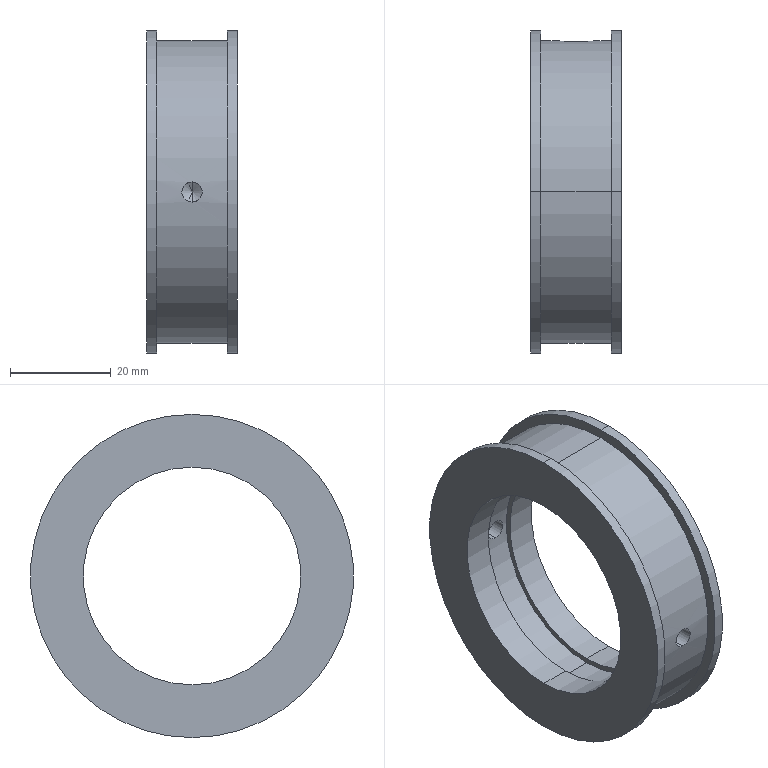Part | SolidWorks | features HoleWzd 3, Fillet 2, Revolution 1 | 1 solid | 31 faces | box 18 x 64 x 64 mm | volume 25166 mm3 | cylinder 18 | plane 7 | torus 2 | spline 2 | cone 2 | commonest cylinder face diameters 4 x4 43.1 x4 64 x4 7.5 x2 45.1 x2 60 x2
STEP:
#1=CARTESIAN_POINT('',(0.6103,28.8,3.75));
#2=VERTEX_POINT('',#1);
#3=CARTESIAN_POINT('',(0.6103,28.8,-3.75));
#4=VERTEX_POINT('',#3);
#5=CARTESIAN_POINT('',(0.6103,28.8,0.));
#6=DIRECTION('',(0.,-1.,0.));
#7=DIRECTION('',(0.,0.,-1.));
#8=AXIS2_PLACEMENT_3D('',#5,#6,#7);
#9=CIRCLE('',#8,3.75);
#10=EDGE_CURVE('',#2,#4,#9,.T.);
#11=ORIENTED_EDGE('',*,*,#10,.F.);
#12=CARTESIAN_POINT('',(0.6103,28.5,3.45));
#13=VERTEX_POINT('',#12);
#14=CARTESIAN_POINT('',(0.6103,28.8,3.45));
#15=DIRECTION('',(1.,0.,0.));
#16=DIRECTION('',(0.,0.,-1.));
#17=AXIS2_PLACEMENT_3D('',#14,#15,#16);
#18=CIRCLE('',#17,0.3);
#19=EDGE_CURVE('',#2,#13,#18,.T.);
#20=ORIENTED_EDGE('',*,*,#19,.T.);
#21=CARTESIAN_POINT('',(0.6103,28.5,-3.45));
#22=VERTEX_POINT('',#21);
#23=CARTESIAN_POINT('',(0.6103,28.5,0.));
#24=DIRECTION('',(0.,1.,0.));
#25=DIRECTION('',(0.,0.,-1.));
#26=AXIS2_PLACEMENT_3D('',#23,#24,#25);
#27=CIRCLE('',#26,3.45);
#28=EDGE_CURVE('',#22,#13,#27,.T.);
#29=ORIENTED_EDGE('',*,*,#28,.F.);
#30=CARTESIAN_POINT('',(0.6103,28.8,-3.45));
#31=DIRECTION('',(-1.,0.,0.));
#32=DIRECTION('',(0.,0.,1.));
#33=AXIS2_PLACEMENT_3D('',#30,#31,#32);
#34=CIRCLE('',#33,0.3);
#35=EDGE_CURVE('',#4,#22,#34,.T.);
#36=ORIENTED_EDGE('',*,*,#35,.F.);
#37=EDGE_LOOP('',(#11,#20,#29,#36));
#38=FACE_OUTER_BOUND('',#37,.T.);
#39=CARTESIAN_POINT('',(0.6103,28.8,0.));
#40=DIRECTION('',(0.,-1.,0.));
#41=DIRECTION('',(0.,0.,-1.));
#42=AXIS2_PLACEMENT_3D('',#39,#40,#41);
#43=TOROIDAL_SURFACE('',#42,3.45,0.3);
#44=ADVANCED_FACE('',(#38),#43,.F.);
#45=CARTESIAN_POINT('',(-0.2424,29.551,-3.652));
#46=VERTEX_POINT('',#45);
#47=CARTESIAN_POINT('',(0.6103,29.537,3.75));
#48=VERTEX_POINT('',#47);
#49=CARTESIAN_POINT('',(-0.2424,29.551,-3.652));
#50=CARTESIAN_POINT('',(-0.4646,29.558,-3.6));
#51=CARTESIAN_POINT('',(-0.6839,29.568,-3.527));
#52=CARTESIAN_POINT('',(-1.101,29.591,-3.345));
#53=CARTESIAN_POINT('',(-1.299,29.605,-3.236));
#54=CARTESIAN_POINT('',(-1.675,29.634,-2.982));
#55=CARTESIAN_POINT('',(-1.854,29.65,-2.836));
#56=CARTESIAN_POINT('',(-2.178,29.682,-2.518));
#57=CARTESIAN_POINT('',(-2.324,29.698,-2.346));
#58=CARTESIAN_POINT('',(-2.586,29.728,-1.974));
#59=CARTESIAN_POINT('',(-2.701,29.742,-1.774));
#60=CARTESIAN_POINT('',(-2.891,29.766,-1.363));
#61=CARTESIAN_POINT('',(-2.967,29.776,-1.149));
#62=CARTESIAN_POINT('',(-3.08,29.792,-0.7059));
#63=CARTESIAN_POINT('',(-3.116,29.797,-0.479));
#64=CARTESIAN_POINT('',(-3.146,29.801,-0.02683));
#65=CARTESIAN_POINT('',(-3.141,29.8,0.2003));
#66=CARTESIAN_POINT('',(-3.089,29.793,0.6567));
#67=CARTESIAN_POINT('',(-3.042,29.786,0.8794));
#68=CARTESIAN_POINT('',(-2.91,29.769,1.312));
#69=CARTESIAN_POINT('',(-2.823,29.757,1.524));
#70=CARTESIAN_POINT('',(-2.613,29.731,1.93));
#71=CARTESIAN_POINT('',(-2.491,29.717,2.121));
#72=CARTESIAN_POINT('',(-2.213,29.686,2.478));
#73=CARTESIAN_POINT('',(-2.056,29.67,2.647));
#74=CARTESIAN_POINT('',(-1.716,29.638,2.95));
#75=CARTESIAN_POINT('',(-1.534,29.623,3.084));
#76=CARTESIAN_POINT('',(-1.147,29.594,3.32));
#77=CARTESIAN_POINT('',(-0.9399,29.581,3.422));
#78=CARTESIAN_POINT('',(-0.5152,29.56,3.584));
#79=CARTESIAN_POINT('',(-0.2972,29.552,3.646));
#80=CARTESIAN_POINT('',(0.1503,29.54,3.729));
#81=CARTESIAN_POINT('',(0.3805,29.537,3.75));
#82=CARTESIAN_POINT('',(0.6103,29.537,3.75));
#83=B_SPLINE_CURVE_WITH_KNOTS('',3,(#49,#50,#51,#52,#53,#54,#55,#56,#57,#58,#59,#60,#61,#62,#63,#64,#65,#66,#67,#68,#69,#70,#71,#72,#73,#74,#75,#76,#77,#78,#79,#80,#81,#82),.UNSPECIFIED.,.F.,.F.,(4,2,2,2,2,2,2,2,2,2,2,2,2,2,2,2,4),(0.01269,0.01337,0.01406,0.01474,0.01543,0.01611,0.0168,0.01748,0.01817,0.01885,0.01954,0.02022,0.02091,0.02159,0.02228,0.02296,0.02365),.UNSPECIFIED.);
#84=EDGE_CURVE('',#46,#48,#83,.T.);
#85=ORIENTED_EDGE('',*,*,#84,.F.);
#86=CARTESIAN_POINT('',(-0.2879,29.749,-3.872));
#87=VERTEX_POINT('',#86);
#88=CARTESIAN_POINT('',(-0.2879,29.551,-3.847));
#89=DIRECTION('',(-0.9734,0.02959,0.2273));
#90=DIRECTION('',(0.2274,0.,0.9738));
#91=AXIS2_PLACEMENT_3D('',#88,#89,#90);
#92=CIRCLE('',#91,0.2);
#93=EDGE_CURVE('',#46,#87,#92,.T.);
#94=ORIENTED_EDGE('',*,*,#93,.T.);
#95=CARTESIAN_POINT('',(1.509,29.749,3.872));
#96=VERTEX_POINT('',#95);
#97=CARTESIAN_POINT('',(1.509,29.749,3.872));
#98=CARTESIAN_POINT('',(1.254,29.741,3.932));
#99=CARTESIAN_POINT('',(0.9958,29.737,3.966));
#100=CARTESIAN_POINT('',(0.4738,29.734,3.983));
#101=CARTESIAN_POINT('',(0.2098,29.737,3.965));
#102=CARTESIAN_POINT('',(-0.3023,29.748,3.878));
#103=CARTESIAN_POINT('',(-0.5513,29.757,3.81));
#104=CARTESIAN_POINT('',(-1.035,29.78,3.624));
#105=CARTESIAN_POINT('',(-1.271,29.795,3.506));
#106=CARTESIAN_POINT('',(-1.707,29.826,3.231));
#107=CARTESIAN_POINT('',(-1.911,29.843,3.072));
#108=CARTESIAN_POINT('',(-2.289,29.878,2.714));
#109=CARTESIAN_POINT('',(-2.459,29.895,2.517));
#110=CARTESIAN_POINT('',(-2.756,29.927,2.096));
#111=CARTESIAN_POINT('',(-2.886,29.943,1.869));
#112=CARTESIAN_POINT('',(-3.098,29.969,1.394));
#113=CARTESIAN_POINT('',(-3.18,29.979,1.149));
#114=CARTESIAN_POINT('',(-3.296,29.994,0.6447));
#115=CARTESIAN_POINT('',(-3.33,29.999,0.3829));
#116=CARTESIAN_POINT('',(-3.346,30.001,-0.135));
#117=CARTESIAN_POINT('',(-3.329,29.999,-0.3927));
#118=CARTESIAN_POINT('',(-3.245,29.987,-0.9056));
#119=CARTESIAN_POINT('',(-3.177,29.979,-1.16));
#120=CARTESIAN_POINT('',(-2.996,29.956,-1.643));
#121=CARTESIAN_POINT('',(-2.882,29.942,-1.876));
#122=CARTESIAN_POINT('',(-2.608,29.911,-2.321));
#123=CARTESIAN_POINT('',(-2.451,29.894,-2.526));
#124=CARTESIAN_POINT('',(-2.1,29.86,-2.904));
#125=CARTESIAN_POINT('',(-1.904,29.842,-3.078));
#126=CARTESIAN_POINT('',(-1.484,29.809,-3.382));
#127=CARTESIAN_POINT('',(-1.261,29.794,-3.512));
#128=CARTESIAN_POINT('',(-0.7903,29.768,-3.727));
#129=CARTESIAN_POINT('',(-0.5411,29.757,-3.813));
#130=CARTESIAN_POINT('',(-0.2879,29.749,-3.872));
#131=B_SPLINE_CURVE_WITH_KNOTS('',3,(#97,#98,#99,#100,#101,#102,#103,#104,#105,#106,#107,#108,#109,#110,#111,#112,#113,#114,#115,#116,#117,#118,#119,#120,#121,#122,#123,#124,#125,#126,#127,#128,#129,#130),.UNSPECIFIED.,.F.,.F.,(4,2,2,2,2,2,2,2,2,2,2,2,2,2,2,2,4),(0.02421,0.025,0.02578,0.02657,0.02735,0.02814,0.02892,0.02971,0.03049,0.03128,0.03206,0.03285,0.03363,0.03442,0.0352,0.03599,0.03677),.UNSPECIFIED.);
#132=EDGE_CURVE('',#96,#87,#131,.T.);
#133=ORIENTED_EDGE('',*,*,#132,.F.);
#134=CARTESIAN_POINT('',(1.463,29.551,3.652));
#135=VERTEX_POINT('',#134);
#136=CARTESIAN_POINT('',(1.509,29.551,3.846));
#137=DIRECTION('',(0.9734,0.02959,-0.2273));
#138=DIRECTION('',(-0.2274,0.,-0.9738));
#139=AXIS2_PLACEMENT_3D('',#136,#137,#138);
#140=CIRCLE('',#139,0.2);
#141=EDGE_CURVE('',#135,#96,#140,.T.);
#142=ORIENTED_EDGE('',*,*,#141,.F.);
#143=CARTESIAN_POINT('',(0.6103,29.537,3.75));
#144=CARTESIAN_POINT('',(0.7544,29.537,3.75));
#145=CARTESIAN_POINT('',(1.041,29.539,3.733));
#146=CARTESIAN_POINT('',(1.323,29.546,3.684));
#147=CARTESIAN_POINT('',(1.463,29.551,3.652));
#148=B_SPLINE_CURVE_WITH_KNOTS('',3,(#143,#144,#145,#146,#147),.UNSPECIFIED.,.F.,.F.,(4,1,4),(0.,0.0004293,0.0008586),.UNSPECIFIED.);
#149=EDGE_CURVE('',#48,#135,#148,.T.);
#150=ORIENTED_EDGE('',*,*,#149,.F.);
#151=EDGE_LOOP('',(#85,#94,#133,#142,#150));
#152=FACE_OUTER_BOUND('',#151,.T.);
#153=CARTESIAN_POINT('',(1.463,29.551,3.652));
#154=CARTESIAN_POINT('',(1.457,29.778,3.653));
#155=CARTESIAN_POINT('',(1.509,29.749,3.872));
#156=CARTESIAN_POINT('',(1.222,29.543,3.708));
#157=CARTESIAN_POINT('',(1.216,29.771,3.709));
#158=CARTESIAN_POINT('',(1.254,29.741,3.932));
#159=CARTESIAN_POINT('',(0.9788,29.538,3.74));
#160=CARTESIAN_POINT('',(0.9757,29.767,3.74));
#161=CARTESIAN_POINT('',(0.9985,29.737,3.966));
#162=CARTESIAN_POINT('',(0.49,29.536,3.756));
#163=CARTESIAN_POINT('',(0.4909,29.765,3.756));
#164=CARTESIAN_POINT('',(0.4835,29.734,3.983));
#165=CARTESIAN_POINT('',(0.2413,29.539,3.74));
#166=CARTESIAN_POINT('',(0.2448,29.767,3.74));
#167=CARTESIAN_POINT('',(0.2217,29.737,3.966));
#168=CARTESIAN_POINT('',(-0.2441,29.55,3.66));
#169=CARTESIAN_POINT('',(-0.237,29.777,3.661));
#170=CARTESIAN_POINT('',(-0.2896,29.748,3.881));
#171=CARTESIAN_POINT('',(-0.4801,29.558,3.596));
#172=CARTESIAN_POINT('',(-0.4712,29.784,3.599));
#173=CARTESIAN_POINT('',(-0.5383,29.757,3.814));
#174=CARTESIAN_POINT('',(-0.9391,29.581,3.424));
#175=CARTESIAN_POINT('',(-0.928,29.804,3.429));
#176=CARTESIAN_POINT('',(-1.022,29.78,3.631));
#177=CARTESIAN_POINT('',(-1.163,29.595,3.313));
#178=CARTESIAN_POINT('',(-1.151,29.817,3.32));
#179=CARTESIAN_POINT('',(-1.257,29.794,3.513));
#180=CARTESIAN_POINT('',(-1.578,29.626,3.055));
#181=CARTESIAN_POINT('',(-1.566,29.844,3.064));
#182=CARTESIAN_POINT('',(-1.695,29.825,3.24));
#183=CARTESIAN_POINT('',(-1.772,29.643,2.907));
#184=CARTESIAN_POINT('',(-1.76,29.859,2.916));
#185=CARTESIAN_POINT('',(-1.899,29.842,3.082));
#186=CARTESIAN_POINT('',(-2.132,29.677,2.57));
#187=CARTESIAN_POINT('',(-2.121,29.89,2.581));
#188=CARTESIAN_POINT('',(-2.278,29.877,2.725));
#189=CARTESIAN_POINT('',(-2.294,29.695,2.384));
#190=CARTESIAN_POINT('',(-2.285,29.905,2.396));
#191=CARTESIAN_POINT('',(-2.449,29.894,2.528));
#192=CARTESIAN_POINT('',(-2.579,29.727,1.988));
#193=CARTESIAN_POINT('',(-2.572,29.934,1.999));
#194=CARTESIAN_POINT('',(-2.749,29.927,2.108));
#195=CARTESIAN_POINT('',(-2.703,29.742,1.774));
#196=CARTESIAN_POINT('',(-2.697,29.948,1.785));
#197=CARTESIAN_POINT('',(-2.88,29.942,1.881));
#198=CARTESIAN_POINT('',(-2.907,29.768,1.325));
#199=CARTESIAN_POINT('',(-2.903,29.971,1.334));
#200=CARTESIAN_POINT('',(-3.094,29.968,1.405));
#201=CARTESIAN_POINT('',(-2.985,29.779,1.093));
#202=CARTESIAN_POINT('',(-2.983,29.981,1.101));
#203=CARTESIAN_POINT('',(-3.177,29.979,1.159));
#204=CARTESIAN_POINT('',(-3.097,29.794,0.6165));
#205=CARTESIAN_POINT('',(-3.096,29.995,0.6213));
#206=CARTESIAN_POINT('',(-3.294,29.994,0.6537));
#207=CARTESIAN_POINT('',(-3.13,29.799,0.3687));
#208=CARTESIAN_POINT('',(-3.129,29.999,0.3714));
#209=CARTESIAN_POINT('',(-3.329,29.999,0.391));
#210=CARTESIAN_POINT('',(-3.146,29.801,-0.1217));
#211=CARTESIAN_POINT('',(-3.146,30.001,-0.1225));
#212=CARTESIAN_POINT('',(-3.346,30.001,-0.129));
#213=CARTESIAN_POINT('',(-3.13,29.799,-0.3657));
#214=CARTESIAN_POINT('',(-3.13,29.999,-0.3686));
#215=CARTESIAN_POINT('',(-3.329,29.999,-0.3878));
#216=CARTESIAN_POINT('',(-3.05,29.788,-0.8512));
#217=CARTESIAN_POINT('',(-3.049,29.989,-0.8574));
#218=CARTESIAN_POINT('',(-3.245,29.988,-0.9027));
#219=CARTESIAN_POINT('',(-2.986,29.779,-1.092));
#220=CARTESIAN_POINT('',(-2.983,29.981,-1.1));
#221=CARTESIAN_POINT('',(-3.177,29.979,-1.158));
#222=CARTESIAN_POINT('',(-2.813,29.756,-1.549));
#223=CARTESIAN_POINT('',(-2.809,29.96,-1.559));
#224=CARTESIAN_POINT('',(-2.996,29.956,-1.643));
#225=CARTESIAN_POINT('',(-2.705,29.743,-1.769));
#226=CARTESIAN_POINT('',(-2.699,29.948,-1.78));
#227=CARTESIAN_POINT('',(-2.882,29.942,-1.876));
#228=CARTESIAN_POINT('',(-2.444,29.711,-2.189));
#229=CARTESIAN_POINT('',(-2.436,29.92,-2.201));
#230=CARTESIAN_POINT('',(-2.607,29.911,-2.322));
#231=CARTESIAN_POINT('',(-2.295,29.695,-2.383));
#232=CARTESIAN_POINT('',(-2.286,29.905,-2.395));
#233=CARTESIAN_POINT('',(-2.45,29.894,-2.527));
#234=CARTESIAN_POINT('',(-1.962,29.661,-2.74));
#235=CARTESIAN_POINT('',(-1.95,29.875,-2.751));
#236=CARTESIAN_POINT('',(-2.099,29.86,-2.905));
#237=CARTESIAN_POINT('',(-1.775,29.643,-2.904));
#238=CARTESIAN_POINT('',(-1.763,29.859,-2.914));
#239=CARTESIAN_POINT('',(-1.902,29.842,-3.08));
#240=CARTESIAN_POINT('',(-1.376,29.61,-3.19));
#241=CARTESIAN_POINT('',(-1.364,29.83,-3.198));
#242=CARTESIAN_POINT('',(-1.482,29.809,-3.383));
#243=CARTESIAN_POINT('',(-1.165,29.595,-3.312));
#244=CARTESIAN_POINT('',(-1.153,29.817,-3.319));
#245=CARTESIAN_POINT('',(-1.259,29.794,-3.512));
#246=CARTESIAN_POINT('',(-0.7184,29.569,-3.515));
#247=CARTESIAN_POINT('',(-0.7081,29.794,-3.519));
#248=CARTESIAN_POINT('',(-0.7893,29.768,-3.728));
#249=CARTESIAN_POINT('',(-0.4816,29.558,-3.596));
#250=CARTESIAN_POINT('',(-0.4729,29.784,-3.598));
#251=CARTESIAN_POINT('',(-0.5398,29.757,-3.813));
#252=CARTESIAN_POINT('',(-0.2424,29.551,-3.652));
#253=CARTESIAN_POINT('',(-0.2359,29.778,-3.653));
#254=CARTESIAN_POINT('',(-0.2879,29.749,-3.872));
#255=(BOUNDED_SURFACE()B_SPLINE_SURFACE(3,2,((#153,#154,#155),(#156,#157,#158),(#159,#160,#161),(#162,#163,#164),(#165,#166,#167),(#168,#169,#170),(#171,#172,#173),(#174,#175,#176),(#177,#178,#179),(#180,#181,#182),(#183,#184,#185),(#186,#187,#188),(#189,#190,#191),(#192,#193,#194),(#195,#196,#197),(#198,#199,#200),(#201,#202,#203),(#204,#205,#206),(#207,#208,#209),(#210,#211,#212),(#213,#214,#215),(#216,#217,#218),(#219,#220,#221),(#222,#223,#224),(#225,#226,#227),(#228,#229,#230),(#231,#232,#233),(#234,#235,#236),(#237,#238,#239),(#240,#241,#242),(#243,#244,#245),(#246,#247,#248),(#249,#250,#251),(#252,#253,#254)),.UNSPECIFIED.,.F.,.F.,.F.)B_SPLINE_SURFACE_WITH_KNOTS((4,2,2,2,2,2,2,2,2,2,2,2,2,2,2,2,4),(3,3),(0.,0.0007725,0.001545,0.002318,0.00309,0.003863,0.004635,0.005408,0.00618,0.006953,0.007725,0.008498,0.00927,0.01004,0.01082,0.01159,0.01236),(0.,1.),.UNSPECIFIED.)GEOMETRIC_REPRESENTATION_ITEM()RATIONAL_B_SPLINE_SURFACE(((1.,0.6612,1.),(1.,0.6597,1.),(1.,0.6588,1.),(1.,0.6584,1.),(1.,0.6589,1.),(1.,0.661,1.),(1.,0.6626,1.),(1.,0.6669,1.),(1.,0.6696,1.),(1.,0.6754,1.),(1.,0.6785,1.),(1.,0.6849,1.),(1.,0.688,1.),(1.,0.694,1.),(1.,0.6967,1.),(1.,0.7014,1.),(1.,0.7033,1.),(1.,0.706,1.),(1.,0.7069,1.),(1.,0.7073,1.),(1.,0.7069,1.),(1.,0.7049,1.),(1.,0.7033,1.),(1.,0.6992,1.),(1.,0.6968,1.),(1.,0.6911,1.),(1.,0.688,1.),(1.,0.6817,1.),(1.,0.6785,1.),(1.,0.6724,1.),(1.,0.6696,1.),(1.,0.6647,1.),(1.,0.6626,1.),(1.,0.6612,1.)))REPRESENTATION_ITEM('')SURFACE());
#256=ADVANCED_FACE('',(#152),#255,.T.);
#257=CARTESIAN_POINT('',(0.6103,-24.798,0.));
#258=VERTEX_POINT('',#257);
#259=CARTESIAN_POINT('',(0.6103,-26.,-2.));
#260=VERTEX_POINT('',#259);
#261=CARTESIAN_POINT('',(0.6103,-26.,-2.));
#262=DIRECTION('',(0.,-0.515,-0.8572));
#263=VECTOR('',#262,1000.);
#264=LINE('',#261,#263);
#265=EDGE_CURVE('',#258,#260,#264,.T.);
#266=ORIENTED_EDGE('',*,*,#265,.F.);
#267=CARTESIAN_POINT('',(0.6103,-26.,2.));
#268=VERTEX_POINT('',#267);
#269=CARTESIAN_POINT('',(0.6103,-26.,2.));
#270=DIRECTION('',(0.,-0.515,0.8572));
#271=VECTOR('',#270,1000.);
#272=LINE('',#269,#271);
#273=EDGE_CURVE('',#258,#268,#272,.T.);
#274=ORIENTED_EDGE('',*,*,#273,.T.);
#275=CARTESIAN_POINT('',(0.6103,-26.,0.));
#276=DIRECTION('',(0.,-1.,0.));
#277=DIRECTION('',(0.,0.,-1.));
#278=AXIS2_PLACEMENT_3D('',#275,#276,#277);
#279=CIRCLE('',#278,2.);
#280=EDGE_CURVE('',#268,#260,#279,.T.);
#281=ORIENTED_EDGE('',*,*,#280,.T.);
#282=EDGE_LOOP('',(#266,#274,#281));
#283=FACE_OUTER_BOUND('',#282,.T.);
#284=CARTESIAN_POINT('',(0.6103,-26.,0.));
#285=DIRECTION('',(0.,-1.,0.));
#286=DIRECTION('',(0.,0.,-1.));
#287=AXIS2_PLACEMENT_3D('',#284,#285,#286);
#288=CONICAL_SURFACE('',#287,2.,1.03);
#289=ADVANCED_FACE('',(#283),#288,.F.);
#290=ORIENTED_EDGE('',*,*,#280,.F.);
#291=CARTESIAN_POINT('',(0.6103,-29.933,2.));
#292=VERTEX_POINT('',#291);
#293=CARTESIAN_POINT('',(0.6103,-30.,2.));
#294=DIRECTION('',(0.,-1.,0.));
#295=VECTOR('',#294,1000.);
#296=LINE('',#293,#295);
#297=EDGE_CURVE('',#268,#292,#296,.T.);
#298=ORIENTED_EDGE('',*,*,#297,.T.);
#299=CARTESIAN_POINT('',(0.6103,-29.933,-2.));
#300=VERTEX_POINT('',#299);
#301=CARTESIAN_POINT('',(0.6103,-29.933,-2.));
#302=CARTESIAN_POINT('',(0.4782,-29.933,-2.));
#303=CARTESIAN_POINT('',(0.3482,-29.934,-1.987));
#304=CARTESIAN_POINT('',(0.0925,-29.937,-1.936));
#305=CARTESIAN_POINT('',(-0.03454,-29.94,-1.898));
#306=CARTESIAN_POINT('',(-0.2768,-29.946,-1.797));
#307=CARTESIAN_POINT('',(-0.3916,-29.95,-1.736));
#308=CARTESIAN_POINT('',(-0.609,-29.958,-1.591));
#309=CARTESIAN_POINT('',(-0.7119,-29.962,-1.506));
#310=CARTESIAN_POINT('',(-0.9886,-29.975,-1.229));
#311=CARTESIAN_POINT('',(-1.138,-29.984,-1.006));
#312=CARTESIAN_POINT('',(-1.337,-29.996,-0.525));
#313=CARTESIAN_POINT('',(-1.39,-30.,-0.2617));
#314=CARTESIAN_POINT('',(-1.39,-30.,0.1298));
#315=CARTESIAN_POINT('',(-1.377,-29.999,0.2623));
#316=CARTESIAN_POINT('',(-1.326,-29.996,0.5189));
#317=CARTESIAN_POINT('',(-1.288,-29.993,0.6436));
#318=CARTESIAN_POINT('',(-1.188,-29.987,0.8858));
#319=CARTESIAN_POINT('',(-1.125,-29.983,1.003));
#320=CARTESIAN_POINT('',(-0.9802,-29.975,1.22));
#321=CARTESIAN_POINT('',(-0.8975,-29.971,1.321));
#322=CARTESIAN_POINT('',(-0.7108,-29.962,1.507));
#323=CARTESIAN_POINT('',(-0.6097,-29.958,1.59));
#324=CARTESIAN_POINT('',(-0.3931,-29.95,1.735));
#325=CARTESIAN_POINT('',(-0.2762,-29.946,1.798));
#326=CARTESIAN_POINT('',(-0.03384,-29.94,1.898));
#327=CARTESIAN_POINT('',(0.09085,-29.937,1.936));
#328=CARTESIAN_POINT('',(0.3472,-29.934,1.987));
#329=CARTESIAN_POINT('',(0.4798,-29.933,2.));
#330=CARTESIAN_POINT('',(0.6103,-29.933,2.));
#331=B_SPLINE_CURVE_WITH_KNOTS('',3,(#301,#302,#303,#304,#305,#306,#307,#308,#309,#310,#311,#312,#313,#314,#315,#316,#317,#318,#319,#320,#321,#322,#323,#324,#325,#326,#327,#328,#329,#330),.UNSPECIFIED.,.F.,.F.,(4,2,2,2,2,2,2,2,2,2,2,2,2,2,4),(0.,0.0003909,0.0007818,0.001173,0.001564,0.002345,0.003127,0.003518,0.003909,0.0043,0.004691,0.005082,0.005473,0.005864,0.006255),.UNSPECIFIED.);
#332=EDGE_CURVE('',#300,#292,#331,.T.);
#333=ORIENTED_EDGE('',*,*,#332,.F.);
#334=CARTESIAN_POINT('',(0.6103,-30.,-2.));
#335=DIRECTION('',(0.,-1.,0.));
#336=VECTOR('',#335,1000.);
#337=LINE('',#334,#336);
#338=EDGE_CURVE('',#260,#300,#337,.T.);
#339=ORIENTED_EDGE('',*,*,#338,.F.);
#340=EDGE_LOOP('',(#290,#298,#333,#339));
#341=FACE_OUTER_BOUND('',#340,.T.);
#342=CARTESIAN_POINT('',(0.6103,-30.,0.));
#343=DIRECTION('',(0.,-1.,0.));
#344=DIRECTION('',(0.,0.,-1.));
#345=AXIS2_PLACEMENT_3D('',#342,#343,#344);
#346=CYLINDRICAL_SURFACE('',#345,2.);
#347=ADVANCED_FACE('',(#341),#346,.F.);
#348=CARTESIAN_POINT('',(0.6103,22.461,-2.));
#349=VERTEX_POINT('',#348);
#350=CARTESIAN_POINT('',(0.6103,22.461,2.));
#351=VERTEX_POINT('',#350);
#352=CARTESIAN_POINT('',(0.6103,22.461,-2.));
#353=CARTESIAN_POINT('',(0.3493,22.461,-2.));
#354=CARTESIAN_POINT('',(0.08608,22.466,-1.948));
#355=CARTESIAN_POINT('',(-0.3953,22.482,-1.748));
#356=CARTESIAN_POINT('',(-0.6184,22.494,-1.599));
#357=CARTESIAN_POINT('',(-0.8951,22.511,-1.323));
#358=CARTESIAN_POINT('',(-0.9796,22.517,-1.22));
#359=CARTESIAN_POINT('',(-1.125,22.528,-1.003));
#360=CARTESIAN_POINT('',(-1.186,22.533,-0.8882));
#361=CARTESIAN_POINT('',(-1.287,22.541,-0.6463));
#362=CARTESIAN_POINT('',(-1.325,22.544,-0.5192));
#363=CARTESIAN_POINT('',(-1.377,22.549,-0.2635));
#364=CARTESIAN_POINT('',(-1.39,22.55,-0.1336));
#365=CARTESIAN_POINT('',(-1.39,22.55,0.1305));
#366=CARTESIAN_POINT('',(-1.377,22.549,0.2608));
#367=CARTESIAN_POINT('',(-1.326,22.544,0.5164));
#368=CARTESIAN_POINT('',(-1.288,22.541,0.6434));
#369=CARTESIAN_POINT('',(-1.188,22.533,0.8857));
#370=CARTESIAN_POINT('',(-1.126,22.528,1.001));
#371=CARTESIAN_POINT('',(-0.9814,22.517,1.218));
#372=CARTESIAN_POINT('',(-0.897,22.511,1.321));
#373=CARTESIAN_POINT('',(-0.6205,22.494,1.598));
#374=CARTESIAN_POINT('',(-0.3977,22.482,1.747));
#375=CARTESIAN_POINT('',(0.08333,22.466,1.947));
#376=CARTESIAN_POINT('',(0.346,22.461,2.));
#377=CARTESIAN_POINT('',(0.6103,22.461,2.));
#378=B_SPLINE_CURVE_WITH_KNOTS('',3,(#352,#353,#354,#355,#356,#357,#358,#359,#360,#361,#362,#363,#364,#365,#366,#367,#368,#369,#370,#371,#372,#373,#374,#375,#376,#377),.UNSPECIFIED.,.F.,.F.,(4,2,2,2,2,2,2,2,2,2,2,2,4),(0.006256,0.007038,0.00782,0.008211,0.008601,0.008992,0.009383,0.009774,0.01017,0.01056,0.01095,0.01173,0.01251),.UNSPECIFIED.);
#379=EDGE_CURVE('',#349,#351,#378,.T.);
#380=ORIENTED_EDGE('',*,*,#379,.F.);
#381=CARTESIAN_POINT('',(0.6103,28.5,-2.));
#382=VERTEX_POINT('',#381);
#383=CARTESIAN_POINT('',(0.6103,28.5,-2.));
#384=DIRECTION('',(0.,1.,0.));
#385=VECTOR('',#384,1000.);
#386=LINE('',#383,#385);
#387=EDGE_CURVE('',#349,#382,#386,.T.);
#388=ORIENTED_EDGE('',*,*,#387,.T.);
#389=CARTESIAN_POINT('',(0.6103,28.5,2.));
#390=VERTEX_POINT('',#389);
#391=CARTESIAN_POINT('',(0.6103,28.5,0.));
#392=DIRECTION('',(0.,1.,0.));
#393=DIRECTION('',(0.,0.,1.));
#394=AXIS2_PLACEMENT_3D('',#391,#392,#393);
#395=CIRCLE('',#394,2.);
#396=EDGE_CURVE('',#382,#390,#395,.T.);
#397=ORIENTED_EDGE('',*,*,#396,.T.);
#398=CARTESIAN_POINT('',(0.6103,28.5,2.));
#399=DIRECTION('',(0.,1.,0.));
#400=VECTOR('',#399,1000.);
#401=LINE('',#398,#400);
#402=EDGE_CURVE('',#351,#390,#401,.T.);
#403=ORIENTED_EDGE('',*,*,#402,.F.);
#404=EDGE_LOOP('',(#380,#388,#397,#403));
#405=FACE_OUTER_BOUND('',#404,.T.);
#406=CARTESIAN_POINT('',(0.6103,28.5,0.));
#407=DIRECTION('',(0.,1.,0.));
#408=DIRECTION('',(0.,0.,1.));
#409=AXIS2_PLACEMENT_3D('',#406,#407,#408);
#410=CYLINDRICAL_SURFACE('',#409,2.);
#411=ADVANCED_FACE('',(#405),#410,.F.);
#412=ORIENTED_EDGE('',*,*,#10,.T.);
#413=CARTESIAN_POINT('',(0.6103,29.537,-3.75));
#414=VERTEX_POINT('',#413);
#415=CARTESIAN_POINT('',(0.6103,30.,-3.75));
#416=DIRECTION('',(0.,1.,0.));
#417=VECTOR('',#416,1000.);
#418=LINE('',#415,#417);
#419=EDGE_CURVE('',#4,#414,#418,.T.);
#420=ORIENTED_EDGE('',*,*,#419,.T.);
#421=CARTESIAN_POINT('',(0.6103,29.537,-3.75));
#422=CARTESIAN_POINT('',(0.4679,29.537,-3.75));
#423=CARTESIAN_POINT('',(0.325,29.538,-3.742));
#424=CARTESIAN_POINT('',(0.03842,29.543,-3.709));
#425=CARTESIAN_POINT('',(-0.1029,29.546,-3.684));
#426=CARTESIAN_POINT('',(-0.2424,29.551,-3.652));
#427=B_SPLINE_CURVE_WITH_KNOTS('',3,(#421,#422,#423,#424,#425,#426),.UNSPECIFIED.,.F.,.F.,(4,2,4),(0.01183,0.01226,0.01269),.UNSPECIFIED.);
#428=EDGE_CURVE('',#414,#46,#427,.T.);
#429=ORIENTED_EDGE('',*,*,#428,.T.);
#430=ORIENTED_EDGE('',*,*,#84,.T.);
#431=CARTESIAN_POINT('',(0.6103,30.,3.75));
#432=DIRECTION('',(0.,1.,0.));
#433=VECTOR('',#432,1000.);
#434=LINE('',#431,#433);
#435=EDGE_CURVE('',#2,#48,#434,.T.);
#436=ORIENTED_EDGE('',*,*,#435,.F.);
#437=EDGE_LOOP('',(#412,#420,#429,#430,#436));
#438=FACE_OUTER_BOUND('',#437,.T.);
#439=CARTESIAN_POINT('',(0.6103,30.,0.));
#440=DIRECTION('',(0.,1.,0.));
#441=DIRECTION('',(0.,0.,1.));
#442=AXIS2_PLACEMENT_3D('',#439,#440,#441);
#443=CYLINDRICAL_SURFACE('',#442,3.75);
#444=ADVANCED_FACE('',(#438),#443,.F.);
#445=CARTESIAN_POINT('',(-2.39,0.,-21.55));
#446=VERTEX_POINT('',#445);
#447=CARTESIAN_POINT('',(-2.39,0.,21.55));
#448=VERTEX_POINT('',#447);
#449=CARTESIAN_POINT('',(-2.39,0.,0.));
#450=DIRECTION('',(-1.,0.,0.));
#451=DIRECTION('',(0.,0.,1.));
#452=AXIS2_PLACEMENT_3D('',#449,#450,#451);
#453=CIRCLE('',#452,21.55);
#454=EDGE_CURVE('',#446,#448,#453,.T.);
#455=ORIENTED_EDGE('',*,*,#454,.F.);
#456=CARTESIAN_POINT('',(-8.39,0.,-21.55));
#457=VERTEX_POINT('',#456);
#458=CARTESIAN_POINT('',(-19.037,0.,-21.55));
#459=DIRECTION('',(-1.,0.,0.));
#460=VECTOR('',#459,1000.);
#461=LINE('',#458,#460);
#462=EDGE_CURVE('',#446,#457,#461,.T.);
#463=ORIENTED_EDGE('',*,*,#462,.T.);
#464=CARTESIAN_POINT('',(-8.39,0.,21.55));
#465=VERTEX_POINT('',#464);
#466=CARTESIAN_POINT('',(-8.39,0.,0.));
#467=DIRECTION('',(-1.,0.,0.));
#468=DIRECTION('',(0.,0.,1.));
#469=AXIS2_PLACEMENT_3D('',#466,#467,#468);
#470=CIRCLE('',#469,21.55);
#471=EDGE_CURVE('',#457,#465,#470,.T.);
#472=ORIENTED_EDGE('',*,*,#471,.T.);
#473=CARTESIAN_POINT('',(-19.037,0.,21.55));
#474=DIRECTION('',(-1.,0.,0.));
#475=VECTOR('',#474,1000.);
#476=LINE('',#473,#475);
#477=EDGE_CURVE('',#448,#465,#476,.T.);
#478=ORIENTED_EDGE('',*,*,#477,.F.);
#479=EDGE_LOOP('',(#455,#463,#472,#478));
#480=FACE_OUTER_BOUND('',#479,.T.);
#481=CARTESIAN_POINT('',(-19.037,0.,0.));
#482=DIRECTION('',(-1.,0.,0.));
#483=DIRECTION('',(0.,0.,1.));
#484=AXIS2_PLACEMENT_3D('',#481,#482,#483);
#485=CYLINDRICAL_SURFACE('',#484,21.55);
#486=ADVANCED_FACE('',(#480),#485,.F.);
#487=CARTESIAN_POINT('',(3.61,0.,-22.55));
#488=VERTEX_POINT('',#487);
#489=CARTESIAN_POINT('',(3.61,0.,22.55));
#490=VERTEX_POINT('',#489);
#491=CARTESIAN_POINT('',(3.61,0.,0.));
#492=DIRECTION('',(-1.,0.,0.));
#493=DIRECTION('',(0.,0.,1.));
#494=AXIS2_PLACEMENT_3D('',#491,#492,#493);
#495=CIRCLE('',#494,22.55);
#496=EDGE_CURVE('',#488,#490,#495,.T.);
#497=ORIENTED_EDGE('',*,*,#496,.F.);
#498=CARTESIAN_POINT('',(-2.39,0.,-22.55));
#499=VERTEX_POINT('',#498);
#500=CARTESIAN_POINT('',(-19.037,0.,-22.55));
#501=DIRECTION('',(-1.,0.,0.));
#502=VECTOR('',#501,1000.);
#503=LINE('',#500,#502);
#504=EDGE_CURVE('',#488,#499,#503,.T.);
#505=ORIENTED_EDGE('',*,*,#504,.T.);
#506=CARTESIAN_POINT('',(-2.39,0.,22.55));
#507=VERTEX_POINT('',#506);
#508=CARTESIAN_POINT('',(-2.39,0.,0.));
#509=DIRECTION('',(-1.,0.,0.));
#510=DIRECTION('',(0.,0.,1.));
#511=AXIS2_PLACEMENT_3D('',#508,#509,#510);
#512=CIRCLE('',#511,22.55);
#513=EDGE_CURVE('',#499,#507,#512,.T.);
#514=ORIENTED_EDGE('',*,*,#513,.T.);
#515=CARTESIAN_POINT('',(-19.037,0.,22.55));
#516=DIRECTION('',(-1.,0.,0.));
#517=VECTOR('',#516,1000.);
#518=LINE('',#515,#517);
#519=EDGE_CURVE('',#490,#507,#518,.T.);
#520=ORIENTED_EDGE('',*,*,#519,.F.);
#521=EDGE_LOOP('',(#497,#505,#514,#520));
#522=FACE_OUTER_BOUND('',#521,.T.);
#523=CARTESIAN_POINT('',(-19.037,0.,0.));
#524=DIRECTION('',(-1.,0.,0.));
#525=DIRECTION('',(0.,0.,1.));
#526=AXIS2_PLACEMENT_3D('',#523,#524,#525);
#527=CYLINDRICAL_SURFACE('',#526,22.55);
#528=ADVANCED_FACE('',(#522),#527,.F.);
#529=CARTESIAN_POINT('',(9.61,0.,-21.55));
#530=VERTEX_POINT('',#529);
#531=CARTESIAN_POINT('',(9.61,0.,21.55));
#532=VERTEX_POINT('',#531);
#533=CARTESIAN_POINT('',(9.61,0.,0.));
#534=DIRECTION('',(-1.,0.,0.));
#535=DIRECTION('',(0.,0.,1.));
#536=AXIS2_PLACEMENT_3D('',#533,#534,#535);
#537=CIRCLE('',#536,21.55);
#538=EDGE_CURVE('',#530,#532,#537,.T.);
#539=ORIENTED_EDGE('',*,*,#538,.F.);
#540=CARTESIAN_POINT('',(3.61,0.,-21.55));
#541=VERTEX_POINT('',#540);
#542=CARTESIAN_POINT('',(-19.037,0.,-21.55));
#543=DIRECTION('',(-1.,0.,0.));
#544=VECTOR('',#543,1000.);
#545=LINE('',#542,#544);
#546=EDGE_CURVE('',#530,#541,#545,.T.);
#547=ORIENTED_EDGE('',*,*,#546,.T.);
#548=CARTESIAN_POINT('',(3.61,0.,21.55));
#549=VERTEX_POINT('',#548);
#550=CARTESIAN_POINT('',(3.61,0.,0.));
#551=DIRECTION('',(-1.,0.,0.));
#552=DIRECTION('',(0.,0.,1.));
#553=AXIS2_PLACEMENT_3D('',#550,#551,#552);
#554=CIRCLE('',#553,21.55);
#555=EDGE_CURVE('',#541,#549,#554,.T.);
#556=ORIENTED_EDGE('',*,*,#555,.T.);
#557=CARTESIAN_POINT('',(-19.037,0.,21.55));
#558=DIRECTION('',(-1.,0.,0.));
#559=VECTOR('',#558,1000.);
#560=LINE('',#557,#559);
#561=EDGE_CURVE('',#532,#549,#560,.T.);
#562=ORIENTED_EDGE('',*,*,#561,.F.);
#563=EDGE_LOOP('',(#539,#547,#556,#562));
#564=FACE_OUTER_BOUND('',#563,.T.);
#565=CARTESIAN_POINT('',(-19.037,0.,0.));
#566=DIRECTION('',(-1.,0.,0.));
#567=DIRECTION('',(0.,0.,1.));
#568=AXIS2_PLACEMENT_3D('',#565,#566,#567);
#569=CYLINDRICAL_SURFACE('',#568,21.55);
#570=ADVANCED_FACE('',(#564),#569,.F.);
#571=CARTESIAN_POINT('',(9.61,0.,32.));
#572=VERTEX_POINT('',#571);
#573=CARTESIAN_POINT('',(9.61,0.,-32.));
#574=VERTEX_POINT('',#573);
#575=CARTESIAN_POINT('',(9.61,0.,0.));
#576=DIRECTION('',(-1.,0.,0.));
#577=DIRECTION('',(0.,0.,1.));
#578=AXIS2_PLACEMENT_3D('',#575,#576,#577);
#579=CIRCLE('',#578,32.);
#580=EDGE_CURVE('',#572,#574,#579,.T.);
#581=ORIENTED_EDGE('',*,*,#580,.T.);
#582=CARTESIAN_POINT('',(7.61,0.,-32.));
#583=VERTEX_POINT('',#582);
#584=CARTESIAN_POINT('',(-19.037,0.,-32.));
#585=DIRECTION('',(-1.,0.,0.));
#586=VECTOR('',#585,1000.);
#587=LINE('',#584,#586);
#588=EDGE_CURVE('',#574,#583,#587,.T.);
#589=ORIENTED_EDGE('',*,*,#588,.T.);
#590=CARTESIAN_POINT('',(7.61,0.,32.));
#591=VERTEX_POINT('',#590);
#592=CARTESIAN_POINT('',(7.61,0.,0.));
#593=DIRECTION('',(-1.,0.,0.));
#594=DIRECTION('',(0.,0.,1.));
#595=AXIS2_PLACEMENT_3D('',#592,#593,#594);
#596=CIRCLE('',#595,32.);
#597=EDGE_CURVE('',#591,#583,#596,.T.);
#598=ORIENTED_EDGE('',*,*,#597,.F.);
#599=CARTESIAN_POINT('',(-19.037,0.,32.));
#600=DIRECTION('',(-1.,0.,0.));
#601=VECTOR('',#600,1000.);
#602=LINE('',#599,#601);
#603=EDGE_CURVE('',#572,#591,#602,.T.);
#604=ORIENTED_EDGE('',*,*,#603,.F.);
#605=EDGE_LOOP('',(#581,#589,#598,#604));
#606=FACE_OUTER_BOUND('',#605,.T.);
#607=CARTESIAN_POINT('',(-19.037,0.,0.));
#608=DIRECTION('',(-1.,0.,0.));
#609=DIRECTION('',(0.,0.,1.));
#610=AXIS2_PLACEMENT_3D('',#607,#608,#609);
#611=CYLINDRICAL_SURFACE('',#610,32.);
#612=ADVANCED_FACE('',(#606),#611,.T.);
#613=ORIENTED_EDGE('',*,*,#132,.T.);
#614=CARTESIAN_POINT('',(-0.2879,29.749,-3.872));
#615=CARTESIAN_POINT('',(-0.03455,29.741,-3.932));
#616=CARTESIAN_POINT('',(0.2272,29.737,-3.966));
#617=CARTESIAN_POINT('',(0.7456,29.734,-3.983));
#618=CARTESIAN_POINT('',(1.003,29.737,-3.965));
#619=CARTESIAN_POINT('',(1.516,29.748,-3.879));
#620=CARTESIAN_POINT('',(1.77,29.757,-3.81));
#621=CARTESIAN_POINT('',(2.253,29.78,-3.626));
#622=CARTESIAN_POINT('',(2.484,29.794,-3.51));
#623=CARTESIAN_POINT('',(2.927,29.826,-3.232));
#624=CARTESIAN_POINT('',(3.131,29.843,-3.073));
#625=CARTESIAN_POINT('',(3.505,29.877,-2.718));
#626=CARTESIAN_POINT('',(3.677,29.895,-2.519));
#627=CARTESIAN_POINT('',(3.977,29.927,-2.096));
#628=CARTESIAN_POINT('',(4.105,29.942,-1.872));
#629=CARTESIAN_POINT('',(4.317,29.968,-1.399));
#630=CARTESIAN_POINT('',(4.401,29.979,-1.149));
#631=CARTESIAN_POINT('',(4.517,29.994,-0.6445));
#632=CARTESIAN_POINT('',(4.55,29.999,-0.3881));
#633=CARTESIAN_POINT('',(4.567,30.001,0.1335));
#634=CARTESIAN_POINT('',(4.549,29.998,0.3946));
#635=CARTESIAN_POINT('',(4.465,29.987,0.9045));
#636=CARTESIAN_POINT('',(4.398,29.979,1.157));
#637=CARTESIAN_POINT('',(4.216,29.956,1.646));
#638=CARTESIAN_POINT('',(4.102,29.942,1.877));
#639=CARTESIAN_POINT('',(3.831,29.911,2.317));
#640=CARTESIAN_POINT('',(3.671,29.894,2.527));
#641=CARTESIAN_POINT('',(3.319,29.86,2.906));
#642=CARTESIAN_POINT('',(3.126,29.842,3.077));
#643=CARTESIAN_POINT('',(2.705,29.809,3.381));
#644=CARTESIAN_POINT('',(2.478,29.794,3.514));
#645=CARTESIAN_POINT('',(2.008,29.768,3.728));
#646=CARTESIAN_POINT('',(1.764,29.757,3.812));
#647=CARTESIAN_POINT('',(1.509,29.749,3.872));
#648=B_SPLINE_CURVE_WITH_KNOTS('',3,(#614,#615,#616,#617,#618,#619,#620,#621,#622,#623,#624,#625,#626,#627,#628,#629,#630,#631,#632,#633,#634,#635,#636,#637,#638,#639,#640,#641,#642,#643,#644,#645,#646,#647),.UNSPECIFIED.,.F.,.F.,(4,2,2,2,2,2,2,2,2,2,2,2,2,2,2,2,4),(0.01165,0.01243,0.01322,0.014,0.01479,0.01557,0.01636,0.01714,0.01793,0.01872,0.0195,0.02029,0.02107,0.02186,0.02264,0.02343,0.02421),.UNSPECIFIED.);
#649=EDGE_CURVE('',#87,#96,#648,.T.);
#650=ORIENTED_EDGE('',*,*,#649,.T.);
#651=EDGE_LOOP('',(#613,#650));
#652=FACE_BOUND('',#651,.T.);
#653=CARTESIAN_POINT('',(7.61,0.,30.));
#654=VERTEX_POINT('',#653);
#655=CARTESIAN_POINT('',(7.61,0.,-30.));
#656=VERTEX_POINT('',#655);
#657=CARTESIAN_POINT('',(7.61,0.,0.));
#658=DIRECTION('',(-1.,0.,0.));
#659=DIRECTION('',(0.,0.,1.));
#660=AXIS2_PLACEMENT_3D('',#657,#658,#659);
#661=CIRCLE('',#660,30.);
#662=EDGE_CURVE('',#654,#656,#661,.T.);
#663=ORIENTED_EDGE('',*,*,#662,.T.);
#664=CARTESIAN_POINT('',(-6.39,0.,-30.));
#665=VERTEX_POINT('',#664);
#666=CARTESIAN_POINT('',(-19.037,0.,-30.));
#667=DIRECTION('',(-1.,0.,0.));
#668=VECTOR('',#667,1000.);
#669=LINE('',#666,#668);
#670=EDGE_CURVE('',#656,#665,#669,.T.);
#671=ORIENTED_EDGE('',*,*,#670,.T.);
#672=CARTESIAN_POINT('',(-6.39,0.,30.));
#673=VERTEX_POINT('',#672);
#674=CARTESIAN_POINT('',(-6.39,0.,0.));
#675=DIRECTION('',(-1.,0.,0.));
#676=DIRECTION('',(0.,0.,1.));
#677=AXIS2_PLACEMENT_3D('',#674,#675,#676);
#678=CIRCLE('',#677,30.);
#679=EDGE_CURVE('',#673,#665,#678,.T.);
#680=ORIENTED_EDGE('',*,*,#679,.F.);
#681=CARTESIAN_POINT('',(-19.037,0.,30.));
#682=DIRECTION('',(-1.,0.,0.));
#683=VECTOR('',#682,1000.);
#684=LINE('',#681,#683);
#685=EDGE_CURVE('',#654,#673,#684,.T.);
#686=ORIENTED_EDGE('',*,*,#685,.F.);
#687=EDGE_LOOP('',(#663,#671,#680,#686));
#688=FACE_OUTER_BOUND('',#687,.T.);
#689=CARTESIAN_POINT('',(-19.037,0.,0.));
#690=DIRECTION('',(-1.,0.,0.));
#691=DIRECTION('',(0.,0.,1.));
#692=AXIS2_PLACEMENT_3D('',#689,#690,#691);
#693=CYLINDRICAL_SURFACE('',#692,30.);
#694=ADVANCED_FACE('',(#652,#688),#693,.T.);
#695=CARTESIAN_POINT('',(-6.39,0.,32.));
#696=VERTEX_POINT('',#695);
#697=CARTESIAN_POINT('',(-6.39,0.,-32.));
#698=VERTEX_POINT('',#697);
#699=CARTESIAN_POINT('',(-6.39,0.,0.));
#700=DIRECTION('',(-1.,0.,0.));
#701=DIRECTION('',(0.,0.,1.));
#702=AXIS2_PLACEMENT_3D('',#699,#700,#701);
#703=CIRCLE('',#702,32.);
#704=EDGE_CURVE('',#696,#698,#703,.T.);
#705=ORIENTED_EDGE('',*,*,#704,.T.);
#706=CARTESIAN_POINT('',(-8.39,0.,-32.));
#707=VERTEX_POINT('',#706);
#708=CARTESIAN_POINT('',(-19.037,0.,-32.));
#709=DIRECTION('',(-1.,0.,0.));
#710=VECTOR('',#709,1000.);
#711=LINE('',#708,#710);
#712=EDGE_CURVE('',#698,#707,#711,.T.);
#713=ORIENTED_EDGE('',*,*,#712,.T.);
#714=CARTESIAN_POINT('',(-8.39,0.,32.));
#715=VERTEX_POINT('',#714);
#716=CARTESIAN_POINT('',(-8.39,0.,0.));
#717=DIRECTION('',(-1.,0.,0.));
#718=DIRECTION('',(0.,0.,1.));
#719=AXIS2_PLACEMENT_3D('',#716,#717,#718);
#720=CIRCLE('',#719,32.);
#721=EDGE_CURVE('',#715,#707,#720,.T.);
#722=ORIENTED_EDGE('',*,*,#721,.F.);
#723=CARTESIAN_POINT('',(-19.037,0.,32.));
#724=DIRECTION('',(-1.,0.,0.));
#725=VECTOR('',#724,1000.);
#726=LINE('',#723,#725);
#727=EDGE_CURVE('',#696,#715,#726,.T.);
#728=ORIENTED_EDGE('',*,*,#727,.F.);
#729=EDGE_LOOP('',(#705,#713,#722,#728));
#730=FACE_OUTER_BOUND('',#729,.T.);
#731=CARTESIAN_POINT('',(-19.037,0.,0.));
#732=DIRECTION('',(-1.,0.,0.));
#733=DIRECTION('',(0.,0.,1.));
#734=AXIS2_PLACEMENT_3D('',#731,#732,#733);
#735=CYLINDRICAL_SURFACE('',#734,32.);
#736=ADVANCED_FACE('',(#730),#735,.T.);
#737=ORIENTED_EDGE('',*,*,#28,.T.);
#738=CARTESIAN_POINT('',(0.6103,28.5,0.));
#739=DIRECTION('',(0.,1.,0.));
#740=DIRECTION('',(0.,0.,-1.));
#741=AXIS2_PLACEMENT_3D('',#738,#739,#740);
#742=CIRCLE('',#741,3.45);
#743=EDGE_CURVE('',#13,#22,#742,.T.);
#744=ORIENTED_EDGE('',*,*,#743,.T.);
#745=EDGE_LOOP('',(#737,#744));
#746=FACE_OUTER_BOUND('',#745,.T.);
#747=CARTESIAN_POINT('',(0.6103,28.5,0.));
#748=DIRECTION('',(0.,1.,0.));
#749=DIRECTION('',(0.,0.,1.));
#750=AXIS2_PLACEMENT_3D('',#747,#748,#749);
#751=CIRCLE('',#750,2.);
#752=EDGE_CURVE('',#390,#382,#751,.T.);
#753=ORIENTED_EDGE('',*,*,#752,.F.);
#754=ORIENTED_EDGE('',*,*,#396,.F.);
#755=EDGE_LOOP('',(#753,#754));
#756=FACE_BOUND('',#755,.T.);
#757=CARTESIAN_POINT('',(0.6103,28.5,0.));
#758=DIRECTION('',(0.,-1.,0.));
#759=DIRECTION('',(0.,0.,-1.));
#760=AXIS2_PLACEMENT_3D('',#757,#758,#759);
#761=PLANE('',#760);
#762=ADVANCED_FACE('',(#746,#756),#761,.F.);
#763=ORIENTED_EDGE('',*,*,#712,.F.);
#764=CARTESIAN_POINT('',(-6.39,0.,0.));
#765=DIRECTION('',(-1.,0.,0.));
#766=DIRECTION('',(0.,0.,1.));
#767=AXIS2_PLACEMENT_3D('',#764,#765,#766);
#768=CIRCLE('',#767,32.);
#769=EDGE_CURVE('',#698,#696,#768,.T.);
#770=ORIENTED_EDGE('',*,*,#769,.T.);
#771=ORIENTED_EDGE('',*,*,#727,.T.);
#772=CARTESIAN_POINT('',(-8.39,0.,0.));
#773=DIRECTION('',(-1.,0.,0.));
#774=DIRECTION('',(0.,0.,1.));
#775=AXIS2_PLACEMENT_3D('',#772,#773,#774);
#776=CIRCLE('',#775,32.);
#777=EDGE_CURVE('',#707,#715,#776,.T.);
#778=ORIENTED_EDGE('',*,*,#777,.F.);
#779=EDGE_LOOP('',(#763,#770,#771,#778));
#780=FACE_OUTER_BOUND('',#779,.T.);
#781=CARTESIAN_POINT('',(-19.037,0.,0.));
#782=DIRECTION('',(-1.,0.,0.));
#783=DIRECTION('',(0.,0.,1.));
#784=AXIS2_PLACEMENT_3D('',#781,#782,#783);
#785=CYLINDRICAL_SURFACE('',#784,32.);
#786=ADVANCED_FACE('',(#780),#785,.T.);
#787=ORIENTED_EDGE('',*,*,#704,.F.);
#788=ORIENTED_EDGE('',*,*,#769,.F.);
#789=EDGE_LOOP('',(#787,#788));
#790=FACE_OUTER_BOUND('',#789,.T.);
#791=ORIENTED_EDGE('',*,*,#679,.T.);
#792=CARTESIAN_POINT('',(-6.39,0.,0.));
#793=DIRECTION('',(-1.,0.,0.));
#794=DIRECTION('',(0.,0.,1.));
#795=AXIS2_PLACEMENT_3D('',#792,#793,#794);
#796=CIRCLE('',#795,30.);
#797=EDGE_CURVE('',#665,#673,#796,.T.);
#798=ORIENTED_EDGE('',*,*,#797,.T.);
#799=EDGE_LOOP('',(#791,#798));
#800=FACE_BOUND('',#799,.T.);
#801=CARTESIAN_POINT('',(-6.39,32.,0.));
#802=DIRECTION('',(-1.,0.,0.));
#803=DIRECTION('',(0.,0.,1.));
#804=AXIS2_PLACEMENT_3D('',#801,#802,#803);
#805=PLANE('',#804);
#806=ADVANCED_FACE('',(#790,#800),#805,.F.);
#807=ORIENTED_EDGE('',*,*,#670,.F.);
#808=CARTESIAN_POINT('',(7.61,0.,0.));
#809=DIRECTION('',(-1.,0.,0.));
#810=DIRECTION('',(0.,0.,1.));
#811=AXIS2_PLACEMENT_3D('',#808,#809,#810);
#812=CIRCLE('',#811,30.);
#813=EDGE_CURVE('',#656,#654,#812,.T.);
#814=ORIENTED_EDGE('',*,*,#813,.T.);
#815=ORIENTED_EDGE('',*,*,#685,.T.);
#816=ORIENTED_EDGE('',*,*,#797,.F.);
#817=EDGE_LOOP('',(#807,#814,#815,#816));
#818=FACE_OUTER_BOUND('',#817,.T.);
#819=ORIENTED_EDGE('',*,*,#332,.T.);
#820=CARTESIAN_POINT('',(0.6103,-29.933,2.));
#821=CARTESIAN_POINT('',(0.8714,-29.933,2.));
#822=CARTESIAN_POINT('',(1.135,-29.937,1.948));
#823=CARTESIAN_POINT('',(1.616,-29.949,1.748));
#824=CARTESIAN_POINT('',(1.839,-29.958,1.599));
#825=CARTESIAN_POINT('',(2.116,-29.971,1.323));
#826=CARTESIAN_POINT('',(2.2,-29.975,1.22));
#827=CARTESIAN_POINT('',(2.346,-29.983,1.003));
#828=CARTESIAN_POINT('',(2.407,-29.987,0.8881));
#829=CARTESIAN_POINT('',(2.508,-29.993,0.6462));
#830=CARTESIAN_POINT('',(2.546,-29.996,0.5191));
#831=CARTESIAN_POINT('',(2.597,-29.999,0.2635));
#832=CARTESIAN_POINT('',(2.61,-30.,0.1336));
#833=CARTESIAN_POINT('',(2.61,-30.,-0.1304));
#834=CARTESIAN_POINT('',(2.598,-29.999,-0.2607));
#835=CARTESIAN_POINT('',(2.547,-29.996,-0.5163));
#836=CARTESIAN_POINT('',(2.509,-29.993,-0.6432));
#837=CARTESIAN_POINT('',(2.408,-29.987,-0.8857));
#838=CARTESIAN_POINT('',(2.347,-29.984,-1.001));
#839=CARTESIAN_POINT('',(2.202,-29.975,-1.218));
#840=CARTESIAN_POINT('',(2.118,-29.971,-1.321));
#841=CARTESIAN_POINT('',(1.933,-29.962,-1.506));
#842=CARTESIAN_POINT('',(1.833,-29.958,-1.588));
#843=CARTESIAN_POINT('',(1.615,-29.95,-1.735));
#844=CARTESIAN_POINT('',(1.498,-29.946,-1.797));
#845=CARTESIAN_POINT('',(1.137,-29.937,-1.947));
#846=CARTESIAN_POINT('',(0.8746,-29.933,-2.));
#847=CARTESIAN_POINT('',(0.6103,-29.933,-2.));
#848=B_SPLINE_CURVE_WITH_KNOTS('',3,(#820,#821,#822,#823,#824,#825,#826,#827,#828,#829,#830,#831,#832,#833,#834,#835,#836,#837,#838,#839,#840,#841,#842,#843,#844,#845,#846,#847),.UNSPECIFIED.,.F.,.F.,(4,2,2,2,2,2,2,2,2,2,2,2,2,4),(0.006255,0.007036,0.007818,0.008209,0.0086,0.00899,0.009381,0.009772,0.01016,0.01055,0.01094,0.01134,0.01173,0.01251),.UNSPECIFIED.);
#849=EDGE_CURVE('',#292,#300,#848,.T.);
#850=ORIENTED_EDGE('',*,*,#849,.T.);
#851=EDGE_LOOP('',(#819,#850));
#852=FACE_BOUND('',#851,.T.);
#853=CARTESIAN_POINT('',(-19.037,0.,0.));
#854=DIRECTION('',(-1.,0.,0.));
#855=DIRECTION('',(0.,0.,1.));
#856=AXIS2_PLACEMENT_3D('',#853,#854,#855);
#857=CYLINDRICAL_SURFACE('',#856,30.);
#858=ADVANCED_FACE('',(#818,#852),#857,.T.);
#859=ORIENTED_EDGE('',*,*,#662,.F.);
#860=ORIENTED_EDGE('',*,*,#813,.F.);
#861=EDGE_LOOP('',(#859,#860));
#862=FACE_BOUND('',#861,.T.);
#863=ORIENTED_EDGE('',*,*,#597,.T.);
#864=CARTESIAN_POINT('',(7.61,0.,0.));
#865=DIRECTION('',(-1.,0.,0.));
#866=DIRECTION('',(0.,0.,1.));
#867=AXIS2_PLACEMENT_3D('',#864,#865,#866);
#868=CIRCLE('',#867,32.);
#869=EDGE_CURVE('',#583,#591,#868,.T.);
#870=ORIENTED_EDGE('',*,*,#869,.T.);
#871=EDGE_LOOP('',(#863,#870));
#872=FACE_OUTER_BOUND('',#871,.T.);
#873=CARTESIAN_POINT('',(7.61,30.,0.));
#874=DIRECTION('',(1.,0.,0.));
#875=DIRECTION('',(0.,0.,-1.));
#876=AXIS2_PLACEMENT_3D('',#873,#874,#875);
#877=PLANE('',#876);
#878=ADVANCED_FACE('',(#862,#872),#877,.F.);
#879=ORIENTED_EDGE('',*,*,#588,.F.);
#880=CARTESIAN_POINT('',(9.61,0.,0.));
#881=DIRECTION('',(-1.,0.,0.));
#882=DIRECTION('',(0.,0.,1.));
#883=AXIS2_PLACEMENT_3D('',#880,#881,#882);
#884=CIRCLE('',#883,32.);
#885=EDGE_CURVE('',#574,#572,#884,.T.);
#886=ORIENTED_EDGE('',*,*,#885,.T.);
#887=ORIENTED_EDGE('',*,*,#603,.T.);
#888=ORIENTED_EDGE('',*,*,#869,.F.);
#889=EDGE_LOOP('',(#879,#886,#887,#888));
#890=FACE_OUTER_BOUND('',#889,.T.);
#891=CARTESIAN_POINT('',(-19.037,0.,0.));
#892=DIRECTION('',(-1.,0.,0.));
#893=DIRECTION('',(0.,0.,1.));
#894=AXIS2_PLACEMENT_3D('',#891,#892,#893);
#895=CYLINDRICAL_SURFACE('',#894,32.);
#896=ADVANCED_FACE('',(#890),#895,.T.);
#897=ORIENTED_EDGE('',*,*,#580,.F.);
#898=ORIENTED_EDGE('',*,*,#885,.F.);
#899=EDGE_LOOP('',(#897,#898));
#900=FACE_OUTER_BOUND('',#899,.T.);
#901=CARTESIAN_POINT('',(9.61,0.,0.));
#902=DIRECTION('',(-1.,0.,0.));
#903=DIRECTION('',(0.,0.,1.));
#904=AXIS2_PLACEMENT_3D('',#901,#902,#903);
#905=CIRCLE('',#904,21.55);
#906=EDGE_CURVE('',#532,#530,#905,.T.);
#907=ORIENTED_EDGE('',*,*,#906,.T.);
#908=ORIENTED_EDGE('',*,*,#538,.T.);
#909=EDGE_LOOP('',(#907,#908));
#910=FACE_BOUND('',#909,.T.);
#911=CARTESIAN_POINT('',(9.61,32.,0.));
#912=DIRECTION('',(-1.,0.,0.));
#913=DIRECTION('',(0.,0.,1.));
#914=AXIS2_PLACEMENT_3D('',#911,#912,#913);
#915=PLANE('',#914);
#916=ADVANCED_FACE('',(#900,#910),#915,.F.);
#917=ORIENTED_EDGE('',*,*,#546,.F.);
#918=ORIENTED_EDGE('',*,*,#906,.F.);
#919=ORIENTED_EDGE('',*,*,#561,.T.);
#920=CARTESIAN_POINT('',(3.61,0.,0.));
#921=DIRECTION('',(-1.,0.,0.));
#922=DIRECTION('',(0.,0.,1.));
#923=AXIS2_PLACEMENT_3D('',#920,#921,#922);
#924=CIRCLE('',#923,21.55);
#925=EDGE_CURVE('',#549,#541,#924,.T.);
#926=ORIENTED_EDGE('',*,*,#925,.T.);
#927=EDGE_LOOP('',(#917,#918,#919,#926));
#928=FACE_OUTER_BOUND('',#927,.T.);
#929=CARTESIAN_POINT('',(-19.037,0.,0.));
#930=DIRECTION('',(-1.,0.,0.));
#931=DIRECTION('',(0.,0.,1.));
#932=AXIS2_PLACEMENT_3D('',#929,#930,#931);
#933=CYLINDRICAL_SURFACE('',#932,21.55);
#934=ADVANCED_FACE('',(#928),#933,.F.);
#935=ORIENTED_EDGE('',*,*,#925,.F.);
#936=ORIENTED_EDGE('',*,*,#555,.F.);
#937=EDGE_LOOP('',(#935,#936));
#938=FACE_BOUND('',#937,.T.);
#939=CARTESIAN_POINT('',(3.61,0.,0.));
#940=DIRECTION('',(-1.,0.,0.));
#941=DIRECTION('',(0.,0.,1.));
#942=AXIS2_PLACEMENT_3D('',#939,#940,#941);
#943=CIRCLE('',#942,22.55);
#944=EDGE_CURVE('',#490,#488,#943,.T.);
#945=ORIENTED_EDGE('',*,*,#944,.T.);
#946=ORIENTED_EDGE('',*,*,#496,.T.);
#947=EDGE_LOOP('',(#945,#946));
#948=FACE_OUTER_BOUND('',#947,.T.);
#949=CARTESIAN_POINT('',(3.61,21.55,0.));
#950=DIRECTION('',(1.,0.,0.));
#951=DIRECTION('',(0.,0.,-1.));
#952=AXIS2_PLACEMENT_3D('',#949,#950,#951);
#953=PLANE('',#952);
#954=ADVANCED_FACE('',(#938,#948),#953,.F.);
#955=ORIENTED_EDGE('',*,*,#504,.F.);
#956=ORIENTED_EDGE('',*,*,#944,.F.);
#957=ORIENTED_EDGE('',*,*,#519,.T.);
#958=CARTESIAN_POINT('',(-2.39,0.,0.));
#959=DIRECTION('',(-1.,0.,0.));
#960=DIRECTION('',(0.,0.,1.));
#961=AXIS2_PLACEMENT_3D('',#958,#959,#960);
#962=CIRCLE('',#961,22.55);
#963=EDGE_CURVE('',#507,#499,#962,.T.);
#964=ORIENTED_EDGE('',*,*,#963,.T.);
#965=EDGE_LOOP('',(#955,#956,#957,#964));
#966=FACE_OUTER_BOUND('',#965,.T.);
#967=CARTESIAN_POINT('',(0.6103,22.461,2.));
#968=CARTESIAN_POINT('',(0.7426,22.461,2.));
#969=CARTESIAN_POINT('',(0.8725,22.462,1.987));
#970=CARTESIAN_POINT('',(1.128,22.467,1.936));
#971=CARTESIAN_POINT('',(1.255,22.47,1.898));
#972=CARTESIAN_POINT('',(1.498,22.478,1.797));
#973=CARTESIAN_POINT('',(1.612,22.483,1.736));
#974=CARTESIAN_POINT('',(1.83,22.494,1.591));
#975=CARTESIAN_POINT('',(1.933,22.5,1.506));
#976=CARTESIAN_POINT('',(2.209,22.517,1.229));
#977=CARTESIAN_POINT('',(2.358,22.529,1.006));
#978=CARTESIAN_POINT('',(2.558,22.545,0.5251));
#979=CARTESIAN_POINT('',(2.61,22.55,0.2618));
#980=CARTESIAN_POINT('',(2.61,22.55,-0.1298));
#981=CARTESIAN_POINT('',(2.597,22.549,-0.2624));
#982=CARTESIAN_POINT('',(2.546,22.544,-0.5189));
#983=CARTESIAN_POINT('',(2.508,22.541,-0.6437));
#984=CARTESIAN_POINT('',(2.408,22.533,-0.8859));
#985=CARTESIAN_POINT('',(2.346,22.528,-1.003));
#986=CARTESIAN_POINT('',(2.201,22.517,-1.22));
#987=CARTESIAN_POINT('',(2.118,22.511,-1.321));
#988=CARTESIAN_POINT('',(1.931,22.5,-1.507));
#989=CARTESIAN_POINT('',(1.83,22.494,-1.59));
#990=CARTESIAN_POINT('',(1.614,22.483,-1.735));
#991=CARTESIAN_POINT('',(1.497,22.478,-1.798));
#992=CARTESIAN_POINT('',(1.255,22.47,-1.898));
#993=CARTESIAN_POINT('',(1.13,22.467,-1.936));
#994=CARTESIAN_POINT('',(0.8735,22.462,-1.987));
#995=CARTESIAN_POINT('',(0.7409,22.461,-2.));
#996=CARTESIAN_POINT('',(0.6103,22.461,-2.));
#997=B_SPLINE_CURVE_WITH_KNOTS('',3,(#967,#968,#969,#970,#971,#972,#973,#974,#975,#976,#977,#978,#979,#980,#981,#982,#983,#984,#985,#986,#987,#988,#989,#990,#991,#992,#993,#994,#995,#996),.UNSPECIFIED.,.F.,.F.,(4,2,2,2,2,2,2,2,2,2,2,2,2,2,4),(0.,0.000391,0.000782,0.001173,0.001564,0.002346,0.003128,0.003519,0.00391,0.004301,0.004692,0.005083,0.005474,0.005865,0.006256),.UNSPECIFIED.);
#998=EDGE_CURVE('',#351,#349,#997,.T.);
#999=ORIENTED_EDGE('',*,*,#998,.T.);
#1000=ORIENTED_EDGE('',*,*,#379,.T.);
#1001=EDGE_LOOP('',(#999,#1000));
#1002=FACE_BOUND('',#1001,.T.);
#1003=CARTESIAN_POINT('',(-19.037,0.,0.));
#1004=DIRECTION('',(-1.,0.,0.));
#1005=DIRECTION('',(0.,0.,1.));
#1006=AXIS2_PLACEMENT_3D('',#1003,#1004,#1005);
#1007=CYLINDRICAL_SURFACE('',#1006,22.55);
#1008=ADVANCED_FACE('',(#966,#1002),#1007,.F.);
#1009=ORIENTED_EDGE('',*,*,#963,.F.);
#1010=ORIENTED_EDGE('',*,*,#513,.F.);
#1011=EDGE_LOOP('',(#1009,#1010));
#1012=FACE_OUTER_BOUND('',#1011,.T.);
#1013=CARTESIAN_POINT('',(-2.39,0.,0.));
#1014=DIRECTION('',(-1.,0.,0.));
#1015=DIRECTION('',(0.,0.,1.));
#1016=AXIS2_PLACEMENT_3D('',#1013,#1014,#1015);
#1017=CIRCLE('',#1016,21.55);
#1018=EDGE_CURVE('',#448,#446,#1017,.T.);
#1019=ORIENTED_EDGE('',*,*,#1018,.T.);
#1020=ORIENTED_EDGE('',*,*,#454,.T.);
#1021=EDGE_LOOP('',(#1019,#1020));
#1022=FACE_BOUND('',#1021,.T.);
#1023=CARTESIAN_POINT('',(-2.39,22.55,0.));
#1024=DIRECTION('',(-1.,0.,0.));
#1025=DIRECTION('',(0.,0.,1.));
#1026=AXIS2_PLACEMENT_3D('',#1023,#1024,#1025);
#1027=PLANE('',#1026);
#1028=ADVANCED_FACE('',(#1012,#1022),#1027,.F.);
#1029=ORIENTED_EDGE('',*,*,#462,.F.);
#1030=ORIENTED_EDGE('',*,*,#1018,.F.);
#1031=ORIENTED_EDGE('',*,*,#477,.T.);
#1032=CARTESIAN_POINT('',(-8.39,0.,0.));
#1033=DIRECTION('',(-1.,0.,0.));
#1034=DIRECTION('',(0.,0.,1.));
#1035=AXIS2_PLACEMENT_3D('',#1032,#1033,#1034);
#1036=CIRCLE('',#1035,21.55);
#1037=EDGE_CURVE('',#465,#457,#1036,.T.);
#1038=ORIENTED_EDGE('',*,*,#1037,.T.);
#1039=EDGE_LOOP('',(#1029,#1030,#1031,#1038));
#1040=FACE_OUTER_BOUND('',#1039,.T.);
#1041=CARTESIAN_POINT('',(-19.037,0.,0.));
#1042=DIRECTION('',(-1.,0.,0.));
#1043=DIRECTION('',(0.,0.,1.));
#1044=AXIS2_PLACEMENT_3D('',#1041,#1042,#1043);
#1045=CYLINDRICAL_SURFACE('',#1044,21.55);
#1046=ADVANCED_FACE('',(#1040),#1045,.F.);
#1047=ORIENTED_EDGE('',*,*,#1037,.F.);
#1048=ORIENTED_EDGE('',*,*,#471,.F.);
#1049=EDGE_LOOP('',(#1047,#1048));
#1050=FACE_BOUND('',#1049,.T.);
#1051=ORIENTED_EDGE('',*,*,#721,.T.);
#1052=ORIENTED_EDGE('',*,*,#777,.T.);
#1053=EDGE_LOOP('',(#1051,#1052));
#1054=FACE_OUTER_BOUND('',#1053,.T.);
#1055=CARTESIAN_POINT('',(-8.39,21.55,0.));
#1056=DIRECTION('',(1.,0.,0.));
#1057=DIRECTION('',(0.,0.,-1.));
#1058=AXIS2_PLACEMENT_3D('',#1055,#1056,#1057);
#1059=PLANE('',#1058);
#1060=ADVANCED_FACE('',(#1050,#1054),#1059,.F.);
#1061=ORIENTED_EDGE('',*,*,#419,.F.);
#1062=CARTESIAN_POINT('',(0.6103,28.8,0.));
#1063=DIRECTION('',(0.,-1.,0.));
#1064=DIRECTION('',(0.,0.,-1.));
#1065=AXIS2_PLACEMENT_3D('',#1062,#1063,#1064);
#1066=CIRCLE('',#1065,3.75);
#1067=EDGE_CURVE('',#4,#2,#1066,.T.);
#1068=ORIENTED_EDGE('',*,*,#1067,.T.);
#1069=ORIENTED_EDGE('',*,*,#435,.T.);
#1070=ORIENTED_EDGE('',*,*,#149,.T.);
#1071=CARTESIAN_POINT('',(1.463,29.551,3.652));
#1072=CARTESIAN_POINT('',(1.687,29.558,3.599));
#1073=CARTESIAN_POINT('',(1.903,29.568,3.528));
#1074=CARTESIAN_POINT('',(2.318,29.591,3.346));
#1075=CARTESIAN_POINT('',(2.519,29.605,3.236));
#1076=CARTESIAN_POINT('',(2.898,29.634,2.981));
#1077=CARTESIAN_POINT('',(3.073,29.65,2.837));
#1078=CARTESIAN_POINT('',(3.396,29.682,2.52));
#1079=CARTESIAN_POINT('',(3.546,29.698,2.345));
#1080=CARTESIAN_POINT('',(3.808,29.728,1.972));
#1081=CARTESIAN_POINT('',(3.921,29.742,1.776));
#1082=CARTESIAN_POINT('',(4.111,29.766,1.364));
#1083=CARTESIAN_POINT('',(4.188,29.776,1.146));
#1084=CARTESIAN_POINT('',(4.301,29.792,0.7048));
#1085=CARTESIAN_POINT('',(4.336,29.797,0.4809));
#1086=CARTESIAN_POINT('',(4.367,29.801,0.02634));
#1087=CARTESIAN_POINT('',(4.362,29.8,-0.2052));
#1088=CARTESIAN_POINT('',(4.309,29.793,-0.6562));
#1089=CARTESIAN_POINT('',(4.263,29.787,-0.8782));
#1090=CARTESIAN_POINT('',(4.13,29.769,-1.315));
#1091=CARTESIAN_POINT('',(4.042,29.757,-1.528));
#1092=CARTESIAN_POINT('',(3.834,29.731,-1.93));
#1093=CARTESIAN_POINT('',(3.711,29.717,-2.121));
#1094=CARTESIAN_POINT('',(3.431,29.686,-2.482));
#1095=CARTESIAN_POINT('',(3.274,29.67,-2.649));
#1096=CARTESIAN_POINT('',(2.937,29.638,-2.95));
#1097=CARTESIAN_POINT('',(2.754,29.622,-3.086));
#1098=CARTESIAN_POINT('',(2.362,29.594,-3.324));
#1099=CARTESIAN_POINT('',(2.158,29.581,-3.423));
#1100=CARTESIAN_POINT('',(1.735,29.56,-3.585));
#1101=CARTESIAN_POINT('',(1.513,29.551,-3.647));
#1102=CARTESIAN_POINT('',(1.063,29.54,-3.73));
#1103=CARTESIAN_POINT('',(0.8374,29.537,-3.75));
#1104=CARTESIAN_POINT('',(0.6103,29.537,-3.75));
#1105=B_SPLINE_CURVE_WITH_KNOTS('',3,(#1071,#1072,#1073,#1074,#1075,#1076,#1077,#1078,#1079,#1080,#1081,#1082,#1083,#1084,#1085,#1086,#1087,#1088,#1089,#1090,#1091,#1092,#1093,#1094,#1095,#1096,#1097,#1098,#1099,#1100,#1101,#1102,#1103,#1104),.UNSPECIFIED.,.F.,.F.,(4,2,2,2,2,2,2,2,2,2,2,2,2,2,2,2,4),(0.0008586,0.001544,0.00223,0.002915,0.0036,0.004286,0.004971,0.005657,0.006342,0.007028,0.007713,0.008399,0.009084,0.00977,0.01046,0.01114,0.01183),.UNSPECIFIED.);
#1106=EDGE_CURVE('',#135,#414,#1105,.T.);
#1107=ORIENTED_EDGE('',*,*,#1106,.T.);
#1108=EDGE_LOOP('',(#1061,#1068,#1069,#1070,#1107));
#1109=FACE_OUTER_BOUND('',#1108,.T.);
#1110=CARTESIAN_POINT('',(0.6103,30.,0.));
#1111=DIRECTION('',(0.,1.,0.));
#1112=DIRECTION('',(0.,0.,1.));
#1113=AXIS2_PLACEMENT_3D('',#1110,#1111,#1112);
#1114=CYLINDRICAL_SURFACE('',#1113,3.75);
#1115=ADVANCED_FACE('',(#1109),#1114,.F.);
#1116=ORIENTED_EDGE('',*,*,#387,.F.);
#1117=ORIENTED_EDGE('',*,*,#998,.F.);
#1118=ORIENTED_EDGE('',*,*,#402,.T.);
#1119=ORIENTED_EDGE('',*,*,#752,.T.);
#1120=EDGE_LOOP('',(#1116,#1117,#1118,#1119));
#1121=FACE_OUTER_BOUND('',#1120,.T.);
#1122=CARTESIAN_POINT('',(0.6103,28.5,0.));
#1123=DIRECTION('',(0.,1.,0.));
#1124=DIRECTION('',(0.,0.,1.));
#1125=AXIS2_PLACEMENT_3D('',#1122,#1123,#1124);
#1126=CYLINDRICAL_SURFACE('',#1125,2.);
#1127=ADVANCED_FACE('',(#1121),#1126,.F.);
#1128=ORIENTED_EDGE('',*,*,#297,.F.);
#1129=CARTESIAN_POINT('',(0.6103,-26.,0.));
#1130=DIRECTION('',(0.,-1.,0.));
#1131=DIRECTION('',(0.,0.,-1.));
#1132=AXIS2_PLACEMENT_3D('',#1129,#1130,#1131);
#1133=CIRCLE('',#1132,2.);
#1134=EDGE_CURVE('',#260,#268,#1133,.T.);
#1135=ORIENTED_EDGE('',*,*,#1134,.F.);
#1136=ORIENTED_EDGE('',*,*,#338,.T.);
#1137=ORIENTED_EDGE('',*,*,#849,.F.);
#1138=EDGE_LOOP('',(#1128,#1135,#1136,#1137));
#1139=FACE_OUTER_BOUND('',#1138,.T.);
#1140=CARTESIAN_POINT('',(0.6103,-30.,0.));
#1141=DIRECTION('',(0.,-1.,0.));
#1142=DIRECTION('',(0.,0.,-1.));
#1143=AXIS2_PLACEMENT_3D('',#1140,#1141,#1142);
#1144=CYLINDRICAL_SURFACE('',#1143,2.);
#1145=ADVANCED_FACE('',(#1139),#1144,.F.);
#1146=ORIENTED_EDGE('',*,*,#273,.F.);
#1147=ORIENTED_EDGE('',*,*,#265,.T.);
#1148=ORIENTED_EDGE('',*,*,#1134,.T.);
#1149=EDGE_LOOP('',(#1146,#1147,#1148));
#1150=FACE_OUTER_BOUND('',#1149,.T.);
#1151=CARTESIAN_POINT('',(0.6103,-26.,0.));
#1152=DIRECTION('',(0.,-1.,0.));
#1153=DIRECTION('',(0.,0.,-1.));
#1154=AXIS2_PLACEMENT_3D('',#1151,#1152,#1153);
#1155=CONICAL_SURFACE('',#1154,2.,1.03);
#1156=ADVANCED_FACE('',(#1150),#1155,.F.);
#1157=ORIENTED_EDGE('',*,*,#93,.F.);
#1158=ORIENTED_EDGE('',*,*,#428,.F.);
#1159=ORIENTED_EDGE('',*,*,#1106,.F.);
#1160=ORIENTED_EDGE('',*,*,#141,.T.);
#1161=ORIENTED_EDGE('',*,*,#649,.F.);
#1162=EDGE_LOOP('',(#1157,#1158,#1159,#1160,#1161));
#1163=FACE_OUTER_BOUND('',#1162,.T.);
#1164=CARTESIAN_POINT('',(-0.2424,29.551,-3.652));
#1165=CARTESIAN_POINT('',(-0.2359,29.778,-3.653));
#1166=CARTESIAN_POINT('',(-0.2879,29.749,-3.872));
#1167=CARTESIAN_POINT('',(-0.003271,29.543,-3.708));
#1168=CARTESIAN_POINT('',(0.002191,29.771,-3.708));
#1169=CARTESIAN_POINT('',(-0.036,29.741,-3.932));
#1170=CARTESIAN_POINT('',(0.245,29.538,-3.74));
#1171=CARTESIAN_POINT('',(0.248,29.767,-3.74));
#1172=CARTESIAN_POINT('',(0.2255,29.737,-3.966));
#1173=CARTESIAN_POINT('',(0.7356,29.536,-3.756));
#1174=CARTESIAN_POINT('',(0.7346,29.765,-3.756));
#1175=CARTESIAN_POINT('',(0.7422,29.734,-3.983));
#1176=CARTESIAN_POINT('',(0.9795,29.539,-3.74));
#1177=CARTESIAN_POINT('',(0.9761,29.767,-3.74));
#1178=CARTESIAN_POINT('',(0.9992,29.737,-3.966));
#1179=CARTESIAN_POINT('',(1.465,29.55,-3.66));
#1180=CARTESIAN_POINT('',(1.458,29.777,-3.661));
#1181=CARTESIAN_POINT('',(1.51,29.748,-3.881));
#1182=CARTESIAN_POINT('',(1.705,29.559,-3.595));
#1183=CARTESIAN_POINT('',(1.696,29.784,-3.598));
#1184=CARTESIAN_POINT('',(1.764,29.757,-3.812));
#1185=CARTESIAN_POINT('',(2.163,29.581,-3.422));
#1186=CARTESIAN_POINT('',(2.152,29.804,-3.427));
#1187=CARTESIAN_POINT('',(2.245,29.78,-3.629));
#1188=CARTESIAN_POINT('',(2.382,29.595,-3.314));
#1189=CARTESIAN_POINT('',(2.37,29.817,-3.321));
#1190=CARTESIAN_POINT('',(2.477,29.794,-3.514));
#1191=CARTESIAN_POINT('',(2.803,29.626,-3.053));
#1192=CARTESIAN_POINT('',(2.79,29.844,-3.061));
#1193=CARTESIAN_POINT('',(2.919,29.825,-3.237));
#1194=CARTESIAN_POINT('',(2.996,29.643,-2.903));
#1195=CARTESIAN_POINT('',(2.984,29.859,-2.913));
#1196=CARTESIAN_POINT('',(3.124,29.842,-3.079));
#1197=CARTESIAN_POINT('',(3.353,29.677,-2.57));
#1198=CARTESIAN_POINT('',(3.342,29.89,-2.581));
#1199=CARTESIAN_POINT('',(3.499,29.877,-2.725));
#1200=CARTESIAN_POINT('',(3.517,29.695,-2.383));
#1201=CARTESIAN_POINT('',(3.507,29.905,-2.394));
#1202=CARTESIAN_POINT('',(3.672,29.894,-2.527));
#1203=CARTESIAN_POINT('',(3.802,29.727,-1.983));
#1204=CARTESIAN_POINT('',(3.795,29.934,-1.995));
#1205=CARTESIAN_POINT('',(3.973,29.927,-2.103));
#1206=CARTESIAN_POINT('',(3.924,29.742,-1.772));
#1207=CARTESIAN_POINT('',(3.919,29.948,-1.783));
#1208=CARTESIAN_POINT('',(4.101,29.942,-1.879));
#1209=CARTESIAN_POINT('',(4.127,29.768,-1.326));
#1210=CARTESIAN_POINT('',(4.123,29.971,-1.335));
#1211=CARTESIAN_POINT('',(4.314,29.968,-1.406));
#1212=CARTESIAN_POINT('',(4.207,29.779,-1.089));
#1213=CARTESIAN_POINT('',(4.205,29.981,-1.097));
#1214=CARTESIAN_POINT('',(4.399,29.979,-1.155));
#1215=CARTESIAN_POINT('',(4.318,29.794,-0.6125));
#1216=CARTESIAN_POINT('',(4.317,29.995,-0.6172));
#1217=CARTESIAN_POINT('',(4.516,29.994,-0.6494));
#1218=CARTESIAN_POINT('',(4.35,29.799,-0.37));
#1219=CARTESIAN_POINT('',(4.35,29.999,-0.3726));
#1220=CARTESIAN_POINT('',(4.55,29.999,-0.3923));
#1221=CARTESIAN_POINT('',(4.366,29.801,0.1235));
#1222=CARTESIAN_POINT('',(4.367,30.001,0.1243));
#1223=CARTESIAN_POINT('',(4.567,30.001,0.131));
#1224=CARTESIAN_POINT('',(4.35,29.799,0.3706));
#1225=CARTESIAN_POINT('',(4.35,29.999,0.3736));
#1226=CARTESIAN_POINT('',(4.549,29.999,0.393));
#1227=CARTESIAN_POINT('',(4.27,29.788,0.8529));
#1228=CARTESIAN_POINT('',(4.269,29.989,0.8591));
#1229=CARTESIAN_POINT('',(4.465,29.987,0.9045));
#1230=CARTESIAN_POINT('',(4.206,29.779,1.092));
#1231=CARTESIAN_POINT('',(4.204,29.981,1.1));
#1232=CARTESIAN_POINT('',(4.398,29.979,1.158));
#1233=CARTESIAN_POINT('',(4.032,29.756,1.554));
#1234=CARTESIAN_POINT('',(4.028,29.96,1.564));
#1235=CARTESIAN_POINT('',(4.215,29.956,1.647));
#1236=CARTESIAN_POINT('',(3.924,29.742,1.773));
#1237=CARTESIAN_POINT('',(3.918,29.948,1.784));
#1238=CARTESIAN_POINT('',(4.101,29.942,1.88));
#1239=CARTESIAN_POINT('',(3.666,29.712,2.188));
#1240=CARTESIAN_POINT('',(3.657,29.92,2.2));
#1241=CARTESIAN_POINT('',(3.829,29.911,2.32));
#1242=CARTESIAN_POINT('',(3.514,29.694,2.386));
#1243=CARTESIAN_POINT('',(3.504,29.905,2.397));
#1244=CARTESIAN_POINT('',(3.669,29.894,2.53));
#1245=CARTESIAN_POINT('',(3.179,29.66,2.743));
#1246=CARTESIAN_POINT('',(3.168,29.874,2.754));
#1247=CARTESIAN_POINT('',(3.316,29.859,2.909));
#1248=CARTESIAN_POINT('',(2.996,29.643,2.904));
#1249=CARTESIAN_POINT('',(2.984,29.859,2.914));
#1250=CARTESIAN_POINT('',(3.123,29.842,3.079));
#1251=CARTESIAN_POINT('',(2.597,29.61,3.19));
#1252=CARTESIAN_POINT('',(2.584,29.83,3.198));
#1253=CARTESIAN_POINT('',(2.702,29.809,3.383));
#1254=CARTESIAN_POINT('',(2.381,29.595,3.315));
#1255=CARTESIAN_POINT('',(2.369,29.816,3.321));
#1256=CARTESIAN_POINT('',(2.476,29.794,3.515));
#1257=CARTESIAN_POINT('',(1.936,29.569,3.516));
#1258=CARTESIAN_POINT('',(1.926,29.794,3.52));
#1259=CARTESIAN_POINT('',(2.007,29.768,3.729));
#1260=CARTESIAN_POINT('',(1.705,29.558,3.595));
#1261=CARTESIAN_POINT('',(1.696,29.784,3.598));
#1262=CARTESIAN_POINT('',(1.763,29.757,3.813));
#1263=CARTESIAN_POINT('',(1.463,29.551,3.652));
#1264=CARTESIAN_POINT('',(1.457,29.778,3.653));
#1265=CARTESIAN_POINT('',(1.509,29.749,3.872));
#1266=(BOUNDED_SURFACE()B_SPLINE_SURFACE(3,2,((#1164,#1165,#1166),(#1167,#1168,#1169),(#1170,#1171,#1172),(#1173,#1174,#1175),(#1176,#1177,#1178),(#1179,#1180,#1181),(#1182,#1183,#1184),(#1185,#1186,#1187),(#1188,#1189,#1190),(#1191,#1192,#1193),(#1194,#1195,#1196),(#1197,#1198,#1199),(#1200,#1201,#1202),(#1203,#1204,#1205),(#1206,#1207,#1208),(#1209,#1210,#1211),(#1212,#1213,#1214),(#1215,#1216,#1217),(#1218,#1219,#1220),(#1221,#1222,#1223),(#1224,#1225,#1226),(#1227,#1228,#1229),(#1230,#1231,#1232),(#1233,#1234,#1235),(#1236,#1237,#1238),(#1239,#1240,#1241),(#1242,#1243,#1244),(#1245,#1246,#1247),(#1248,#1249,#1250),(#1251,#1252,#1253),(#1254,#1255,#1256),(#1257,#1258,#1259),(#1260,#1261,#1262),(#1263,#1264,#1265)),.UNSPECIFIED.,.F.,.F.,.T.)B_SPLINE_SURFACE_WITH_KNOTS((4,2,2,2,2,2,2,2,2,2,2,2,2,2,2,2,4),(3,3),(0.01236,0.01313,0.01391,0.01468,0.01545,0.01622,0.017,0.01777,0.01854,0.01931,0.02009,0.02086,0.02163,0.0224,0.02318,0.02395,0.02472),(0.,1.),.UNSPECIFIED.)GEOMETRIC_REPRESENTATION_ITEM()RATIONAL_B_SPLINE_SURFACE(((1.,0.6612,1.),(1.,0.6597,1.),(1.,0.6588,1.),(1.,0.6584,1.),(1.,0.6589,1.),(1.,0.661,1.),(1.,0.6627,1.),(1.,0.667,1.),(1.,0.6696,1.),(1.,0.6754,1.),(1.,0.6785,1.),(1.,0.6849,1.),(1.,0.6881,1.),(1.,0.694,1.),(1.,0.6967,1.),(1.,0.7014,1.),(1.,0.7033,1.),(1.,0.706,1.),(1.,0.7069,1.),(1.,0.7073,1.),(1.,0.7068,1.),(1.,0.7049,1.),(1.,0.7033,1.),(1.,0.6992,1.),(1.,0.6967,1.),(1.,0.6911,1.),(1.,0.688,1.),(1.,0.6817,1.),(1.,0.6785,1.),(1.,0.6724,1.),(1.,0.6695,1.),(1.,0.6647,1.),(1.,0.6626,1.),(1.,0.6612,1.)))REPRESENTATION_ITEM('')SURFACE());
#1267=ADVANCED_FACE('',(#1163),#1266,.T.);
#1268=ORIENTED_EDGE('',*,*,#19,.F.);
#1269=ORIENTED_EDGE('',*,*,#1067,.F.);
#1270=ORIENTED_EDGE('',*,*,#35,.T.);
#1271=ORIENTED_EDGE('',*,*,#743,.F.);
#1272=EDGE_LOOP('',(#1268,#1269,#1270,#1271));
#1273=FACE_OUTER_BOUND('',#1272,.T.);
#1274=CARTESIAN_POINT('',(0.6103,28.8,0.));
#1275=DIRECTION('',(0.,-1.,0.));
#1276=DIRECTION('',(0.,0.,-1.));
#1277=AXIS2_PLACEMENT_3D('',#1274,#1275,#1276);
#1278=TOROIDAL_SURFACE('',#1277,3.45,0.3);
#1279=ADVANCED_FACE('',(#1273),#1278,.F.);
#1280=CLOSED_SHELL('',(#44,#256,#289,#347,#411,#444,#486,#528,#570,#612,#694,#736,#762,#786,#806,#858,#878,#896,#916,#934,#954,#1008,#1028,#1046,#1060,#1115,#1127,#1145,#1156,#1267,#1279));
#1281=MANIFOLD_SOLID_BREP('',#1280);
#1282=CARTESIAN_POINT('',(0.,0.,0.));
#1283=DIRECTION('',(0.,0.,1.));
#1284=DIRECTION('',(1.,0.,0.));
#1285=AXIS2_PLACEMENT_3D('',#1282,#1283,#1284);
#1286=(LENGTH_UNIT()NAMED_UNIT(*)SI_UNIT(.MILLI.,.METRE.));
#1287=UNCERTAINTY_MEASURE_WITH_UNIT(LENGTH_MEASURE(0.00001),#1286,'','');
#1288=(NAMED_UNIT(*)PLANE_ANGLE_UNIT()SI_UNIT($,.RADIAN.));
#1289=(NAMED_UNIT(*)SI_UNIT($,.STERADIAN.)SOLID_ANGLE_UNIT());
#1290=(GEOMETRIC_REPRESENTATION_CONTEXT(3)GLOBAL_UNCERTAINTY_ASSIGNED_CONTEXT((#1287))GLOBAL_UNIT_ASSIGNED_CONTEXT((#1286,#1288,#1289))REPRESENTATION_CONTEXT('',''));
#1291=ADVANCED_BREP_SHAPE_REPRESENTATION('',(#1281,#1285),#1290);